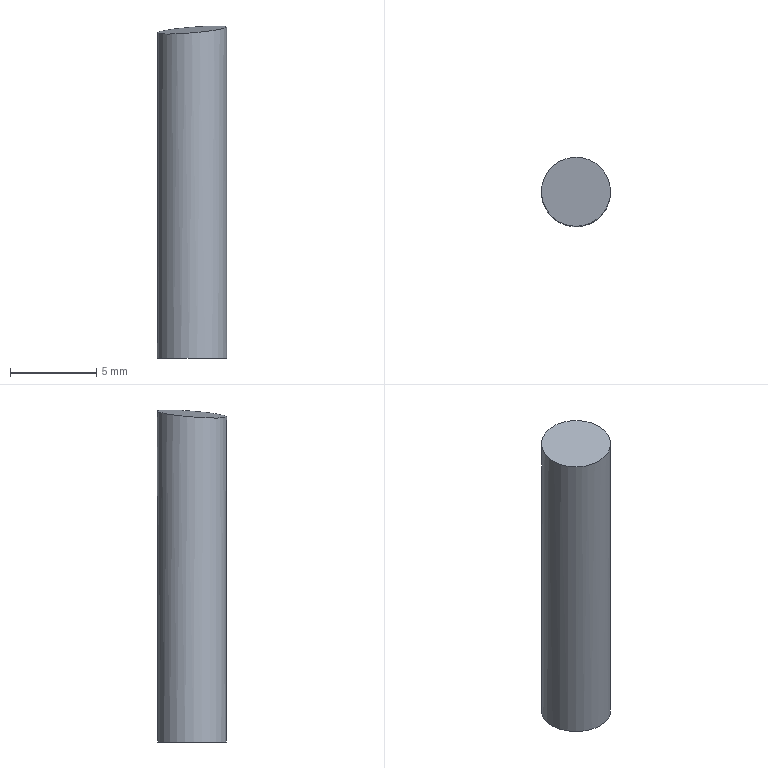Part | NX | features solid 2 | 1 solid | 3 faces | box 4 x 4 x 19.208 mm | volume 238.45 mm3 | plane 2 | cylinder 1 | commonest cylinder face diameters 4 x1
STEP:
#1=CARTESIAN_POINT('',(777.56,8.052,-2.));
#2=VERTEX_POINT('',#1);
#3=CARTESIAN_POINT('',(775.56,8.052,-2.));
#4=DIRECTION('',(0.,0.,1.));
#5=DIRECTION('',(1.,0.,0.));
#6=AXIS2_PLACEMENT_3D('',#3,#4,#5);
#7=CIRCLE('',#6,2.);
#8=EDGE_CURVE('',#2,#2,#7,.T.);
#9=ORIENTED_EDGE('',*,*,#8,.F.);
#10=EDGE_LOOP('',(#9));
#11=FACE_BOUND('',#10,.T.);
#12=CARTESIAN_POINT('',(775.56,8.052,-2.));
#13=DIRECTION('',(0.,0.,-1.));
#14=DIRECTION('',(-1.,0.,0.));
#15=AXIS2_PLACEMENT_3D('',#12,#13,#14);
#16=PLANE('',#15);
#17=ADVANCED_FACE('',(#11),#16,.T.);
#18=CARTESIAN_POINT('',(774.14,6.644,16.743));
#19=VERTEX_POINT('',#18);
#20=CARTESIAN_POINT('',(775.56,8.052,16.975));
#21=DIRECTION('',(0.08207,0.08131,-0.9933));
#22=DIRECTION('',(-0.7057,-0.6991,-0.1155));
#23=AXIS2_PLACEMENT_3D('',#20,#21,#22);
#24=ELLIPSE('',#23,2.013,2.);
#25=EDGE_CURVE('',#19,#19,#24,.T.);
#26=ORIENTED_EDGE('',*,*,#25,.F.);
#27=EDGE_LOOP('',(#26));
#28=FACE_BOUND('',#27,.T.);
#29=CARTESIAN_POINT('',(769.017,-96.065,7.912));
#30=DIRECTION('',(0.08207,0.08131,-0.9933));
#31=DIRECTION('',(0.9966,-0.01117,0.08143));
#32=AXIS2_PLACEMENT_3D('',#29,#30,#31);
#33=PLANE('',#32);
#34=ADVANCED_FACE('',(#28),#33,.F.);
#35=ORIENTED_EDGE('',*,*,#8,.T.);
#36=EDGE_LOOP('',(#35));
#37=FACE_BOUND('',#36,.T.);
#38=ORIENTED_EDGE('',*,*,#25,.T.);
#39=EDGE_LOOP('',(#38));
#40=FACE_BOUND('',#39,.T.);
#41=CARTESIAN_POINT('',(775.56,8.052,18.));
#42=DIRECTION('',(0.,0.,-1.));
#43=DIRECTION('',(-1.,0.,0.));
#44=AXIS2_PLACEMENT_3D('',#41,#42,#43);
#45=CYLINDRICAL_SURFACE('',#44,2.);
#46=ADVANCED_FACE('',(#37,#40),#45,.T.);
#47=CLOSED_SHELL('',(#17,#34,#46));
#48=MANIFOLD_SOLID_BREP('',#47);
#49=(LENGTH_UNIT()NAMED_UNIT(*)SI_UNIT(.MILLI.,.METRE.));
#50=UNCERTAINTY_MEASURE_WITH_UNIT(LENGTH_MEASURE(0.00001),#49,'','');
#51=(NAMED_UNIT(*)PLANE_ANGLE_UNIT()SI_UNIT($,.RADIAN.));
#52=(NAMED_UNIT(*)SI_UNIT($,.STERADIAN.)SOLID_ANGLE_UNIT());
#53=(GEOMETRIC_REPRESENTATION_CONTEXT(3)GLOBAL_UNCERTAINTY_ASSIGNED_CONTEXT((#50))GLOBAL_UNIT_ASSIGNED_CONTEXT((#49,#51,#52))REPRESENTATION_CONTEXT('',''));
#54=ADVANCED_BREP_SHAPE_REPRESENTATION('',(#48),#53);